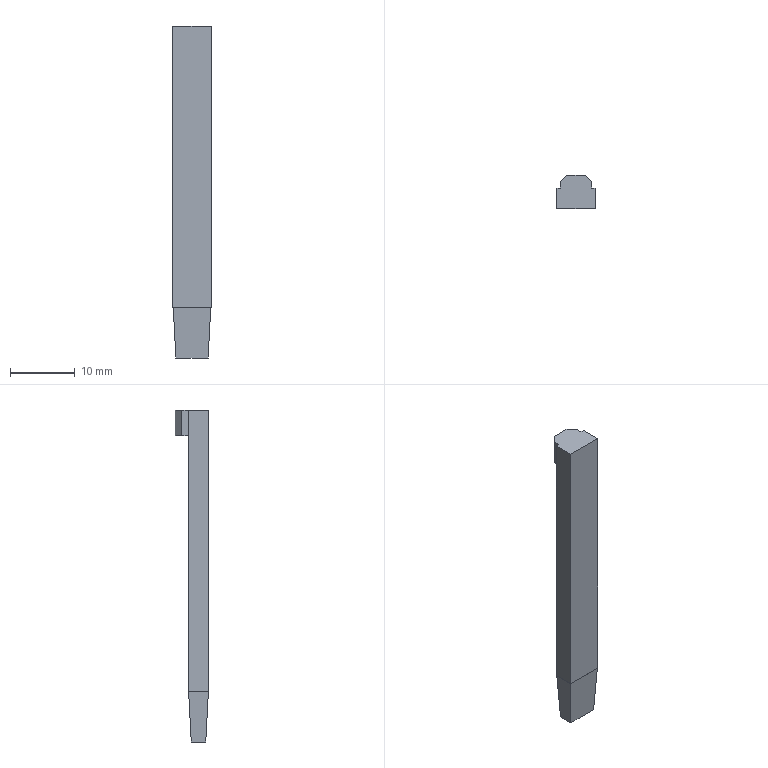Part | Creo | 1 solid | 21 faces | box 5.891 x 5.155 x 51.155 mm | volume 951.101 mm3 | plane 21
STEP:
#1=CARTESIAN_POINT('',(0.,0.,0.));
#2=DIRECTION('',(0.,0.,1.));
#3=DIRECTION('',(1.,0.,0.));
#4=AXIS2_PLACEMENT_3D('',#1,#2,#3);
#5=CARTESIAN_POINT('',(-32.42,12.973,85.91));
#6=VERTEX_POINT('',#5);
#7=CARTESIAN_POINT('',(-32.42,12.973,42.593));
#8=VERTEX_POINT('',#7);
#9=CARTESIAN_POINT('',(-32.42,12.973,85.91));
#10=DIRECTION('',(0.,0.,-1.));
#11=VECTOR('',#10,43.316);
#12=LINE('',#9,#11);
#13=EDGE_CURVE('',#6,#8,#12,.T.);
#14=ORIENTED_EDGE('',*,*,#13,.F.);
#15=CARTESIAN_POINT('',(-26.529,12.973,85.91));
#16=VERTEX_POINT('',#15);
#17=CARTESIAN_POINT('',(-32.42,12.973,85.91));
#18=DIRECTION('',(1.,0.,0.));
#19=VECTOR('',#18,5.891);
#20=LINE('',#17,#19);
#21=EDGE_CURVE('',#6,#16,#20,.T.);
#22=ORIENTED_EDGE('',*,*,#21,.T.);
#23=CARTESIAN_POINT('',(-26.529,12.973,42.593));
#24=VERTEX_POINT('',#23);
#25=CARTESIAN_POINT('',(-26.529,12.973,85.91));
#26=DIRECTION('',(0.,0.,-1.));
#27=VECTOR('',#26,43.316);
#28=LINE('',#25,#27);
#29=EDGE_CURVE('',#16,#24,#28,.T.);
#30=ORIENTED_EDGE('',*,*,#29,.T.);
#31=CARTESIAN_POINT('',(-26.529,12.973,42.593));
#32=DIRECTION('',(-1.,0.,0.));
#33=VECTOR('',#32,5.891);
#34=LINE('',#31,#33);
#35=EDGE_CURVE('',#24,#8,#34,.T.);
#36=ORIENTED_EDGE('',*,*,#35,.T.);
#37=EDGE_LOOP('',(#14,#22,#30,#36));
#38=FACE_OUTER_BOUND('',#37,.F.);
#39=CARTESIAN_POINT('',(-29.474,12.973,14.755));
#40=DIRECTION('',(0.,-1.,0.));
#41=DIRECTION('',(0.,0.,-1.));
#42=AXIS2_PLACEMENT_3D('',#39,#40,#41);
#43=PLANE('',#42);
#44=ADVANCED_FACE('',(#38),#43,.T.);
#45=CARTESIAN_POINT('',(-32.42,16.128,85.91));
#46=VERTEX_POINT('',#45);
#47=CARTESIAN_POINT('',(-32.42,16.128,42.593));
#48=VERTEX_POINT('',#47);
#49=CARTESIAN_POINT('',(-32.42,16.128,85.91));
#50=DIRECTION('',(0.,0.,-1.));
#51=VECTOR('',#50,43.316);
#52=LINE('',#49,#51);
#53=EDGE_CURVE('',#46,#48,#52,.T.);
#54=ORIENTED_EDGE('',*,*,#53,.F.);
#55=CARTESIAN_POINT('',(-32.42,16.128,85.91));
#56=DIRECTION('',(0.,-1.,0.));
#57=VECTOR('',#56,3.155);
#58=LINE('',#55,#57);
#59=EDGE_CURVE('',#46,#6,#58,.T.);
#60=ORIENTED_EDGE('',*,*,#59,.T.);
#61=ORIENTED_EDGE('',*,*,#13,.T.);
#62=CARTESIAN_POINT('',(-32.42,12.973,42.593));
#63=DIRECTION('',(0.,1.,0.));
#64=VECTOR('',#63,3.155);
#65=LINE('',#62,#64);
#66=EDGE_CURVE('',#8,#48,#65,.T.);
#67=ORIENTED_EDGE('',*,*,#66,.T.);
#68=EDGE_LOOP('',(#54,#60,#61,#67));
#69=FACE_OUTER_BOUND('',#68,.F.);
#70=CARTESIAN_POINT('',(-32.42,14.551,14.755));
#71=DIRECTION('',(-1.,0.,0.));
#72=DIRECTION('',(0.,0.,1.));
#73=AXIS2_PLACEMENT_3D('',#70,#71,#72);
#74=PLANE('',#73);
#75=ADVANCED_FACE('',(#69),#74,.T.);
#76=CARTESIAN_POINT('',(-26.529,16.128,85.91));
#77=VERTEX_POINT('',#76);
#78=CARTESIAN_POINT('',(-26.529,16.128,42.593));
#79=VERTEX_POINT('',#78);
#80=CARTESIAN_POINT('',(-26.529,16.128,85.91));
#81=DIRECTION('',(0.,0.,-1.));
#82=VECTOR('',#81,43.316);
#83=LINE('',#80,#82);
#84=EDGE_CURVE('',#77,#79,#83,.T.);
#85=ORIENTED_EDGE('',*,*,#84,.F.);
#86=CARTESIAN_POINT('',(-27.079,16.128,85.91));
#87=VERTEX_POINT('',#86);
#88=CARTESIAN_POINT('',(-26.529,16.128,85.91));
#89=DIRECTION('',(-1.,0.,0.));
#90=VECTOR('',#89,0.55);
#91=LINE('',#88,#90);
#92=EDGE_CURVE('',#77,#87,#91,.T.);
#93=ORIENTED_EDGE('',*,*,#92,.T.);
#94=CARTESIAN_POINT('',(-27.079,16.128,81.91));
#95=VERTEX_POINT('',#94);
#96=CARTESIAN_POINT('',(-27.079,16.128,81.91));
#97=DIRECTION('',(0.,0.,1.));
#98=VECTOR('',#97,4.);
#99=LINE('',#96,#98);
#100=EDGE_CURVE('',#95,#87,#99,.T.);
#101=ORIENTED_EDGE('',*,*,#100,.F.);
#102=CARTESIAN_POINT('',(-31.87,16.128,81.91));
#103=VERTEX_POINT('',#102);
#104=CARTESIAN_POINT('',(-31.87,16.128,81.91));
#105=DIRECTION('',(1.,0.,0.));
#106=VECTOR('',#105,4.791);
#107=LINE('',#104,#106);
#108=EDGE_CURVE('',#103,#95,#107,.T.);
#109=ORIENTED_EDGE('',*,*,#108,.F.);
#110=CARTESIAN_POINT('',(-31.87,16.128,85.91));
#111=VERTEX_POINT('',#110);
#112=CARTESIAN_POINT('',(-31.87,16.128,85.91));
#113=DIRECTION('',(0.,0.,-1.));
#114=VECTOR('',#113,4.);
#115=LINE('',#112,#114);
#116=EDGE_CURVE('',#111,#103,#115,.T.);
#117=ORIENTED_EDGE('',*,*,#116,.F.);
#118=CARTESIAN_POINT('',(-31.87,16.128,85.91));
#119=DIRECTION('',(-1.,0.,0.));
#120=VECTOR('',#119,0.55);
#121=LINE('',#118,#120);
#122=EDGE_CURVE('',#111,#46,#121,.T.);
#123=ORIENTED_EDGE('',*,*,#122,.T.);
#124=ORIENTED_EDGE('',*,*,#53,.T.);
#125=CARTESIAN_POINT('',(-32.42,16.128,42.593));
#126=DIRECTION('',(1.,0.,0.));
#127=VECTOR('',#126,5.891);
#128=LINE('',#125,#127);
#129=EDGE_CURVE('',#48,#79,#128,.T.);
#130=ORIENTED_EDGE('',*,*,#129,.T.);
#131=EDGE_LOOP('',(#85,#93,#101,#109,#117,#123,#124,#130));
#132=FACE_OUTER_BOUND('',#131,.F.);
#133=CARTESIAN_POINT('',(-29.474,16.128,14.755));
#134=DIRECTION('',(0.,1.,0.));
#135=DIRECTION('',(0.,0.,1.));
#136=AXIS2_PLACEMENT_3D('',#133,#134,#135);
#137=PLANE('',#136);
#138=ADVANCED_FACE('',(#132),#137,.T.);
#139=ORIENTED_EDGE('',*,*,#29,.F.);
#140=CARTESIAN_POINT('',(-26.529,12.973,85.91));
#141=DIRECTION('',(0.,1.,0.));
#142=VECTOR('',#141,3.155);
#143=LINE('',#140,#142);
#144=EDGE_CURVE('',#16,#77,#143,.T.);
#145=ORIENTED_EDGE('',*,*,#144,.T.);
#146=ORIENTED_EDGE('',*,*,#84,.T.);
#147=CARTESIAN_POINT('',(-26.529,16.128,42.593));
#148=DIRECTION('',(0.,-1.,0.));
#149=VECTOR('',#148,3.155);
#150=LINE('',#147,#149);
#151=EDGE_CURVE('',#79,#24,#150,.T.);
#152=ORIENTED_EDGE('',*,*,#151,.T.);
#153=EDGE_LOOP('',(#139,#145,#146,#152));
#154=FACE_OUTER_BOUND('',#153,.F.);
#155=CARTESIAN_POINT('',(-26.529,14.551,14.755));
#156=DIRECTION('',(1.,0.,0.));
#157=DIRECTION('',(0.,0.,-1.));
#158=AXIS2_PLACEMENT_3D('',#155,#156,#157);
#159=PLANE('',#158);
#160=ADVANCED_FACE('',(#154),#159,.T.);
#161=CARTESIAN_POINT('',(-27.079,17.128,85.91));
#162=VERTEX_POINT('',#161);
#163=CARTESIAN_POINT('',(-27.079,16.128,85.91));
#164=DIRECTION('',(0.,1.,0.));
#165=VECTOR('',#164,1.);
#166=LINE('',#163,#165);
#167=EDGE_CURVE('',#87,#162,#166,.T.);
#168=ORIENTED_EDGE('',*,*,#167,.F.);
#169=ORIENTED_EDGE('',*,*,#92,.F.);
#170=ORIENTED_EDGE('',*,*,#144,.F.);
#171=ORIENTED_EDGE('',*,*,#21,.F.);
#172=ORIENTED_EDGE('',*,*,#59,.F.);
#173=ORIENTED_EDGE('',*,*,#122,.F.);
#174=CARTESIAN_POINT('',(-31.87,17.128,85.91));
#175=VERTEX_POINT('',#174);
#176=CARTESIAN_POINT('',(-31.87,17.128,85.91));
#177=DIRECTION('',(0.,-1.,0.));
#178=VECTOR('',#177,1.);
#179=LINE('',#176,#178);
#180=EDGE_CURVE('',#175,#111,#179,.T.);
#181=ORIENTED_EDGE('',*,*,#180,.F.);
#182=CARTESIAN_POINT('',(-30.87,18.128,85.91));
#183=VERTEX_POINT('',#182);
#184=CARTESIAN_POINT('',(-30.87,18.128,85.91));
#185=DIRECTION('',(-0.7071,-0.7071,0.));
#186=VECTOR('',#185,1.414);
#187=LINE('',#184,#186);
#188=EDGE_CURVE('',#183,#175,#187,.T.);
#189=ORIENTED_EDGE('',*,*,#188,.F.);
#190=CARTESIAN_POINT('',(-28.079,18.128,85.91));
#191=VERTEX_POINT('',#190);
#192=CARTESIAN_POINT('',(-28.079,18.128,85.91));
#193=DIRECTION('',(-1.,0.,0.));
#194=VECTOR('',#193,2.791);
#195=LINE('',#192,#194);
#196=EDGE_CURVE('',#191,#183,#195,.T.);
#197=ORIENTED_EDGE('',*,*,#196,.F.);
#198=CARTESIAN_POINT('',(-27.079,17.128,85.91));
#199=DIRECTION('',(-0.7071,0.7071,0.));
#200=VECTOR('',#199,1.414);
#201=LINE('',#198,#200);
#202=EDGE_CURVE('',#162,#191,#201,.T.);
#203=ORIENTED_EDGE('',*,*,#202,.F.);
#204=EDGE_LOOP('',(#168,#169,#170,#171,#172,#173,#181,#189,#197,#203));
#205=FACE_OUTER_BOUND('',#204,.F.);
#206=CARTESIAN_POINT('',(62.144,-0.4125,85.91));
#207=DIRECTION('',(0.,0.,1.));
#208=DIRECTION('',(0.,1.,0.));
#209=AXIS2_PLACEMENT_3D('',#206,#207,#208);
#210=PLANE('',#209);
#211=ADVANCED_FACE('',(#205),#210,.T.);
#212=CARTESIAN_POINT('',(-27.079,17.128,81.91));
#213=VERTEX_POINT('',#212);
#214=CARTESIAN_POINT('',(-27.079,17.128,81.91));
#215=DIRECTION('',(0.,-1.,0.));
#216=VECTOR('',#215,1.);
#217=LINE('',#214,#216);
#218=EDGE_CURVE('',#213,#95,#217,.T.);
#219=ORIENTED_EDGE('',*,*,#218,.T.);
#220=ORIENTED_EDGE('',*,*,#100,.T.);
#221=ORIENTED_EDGE('',*,*,#167,.T.);
#222=CARTESIAN_POINT('',(-27.079,17.128,85.91));
#223=DIRECTION('',(0.,0.,-1.));
#224=VECTOR('',#223,4.);
#225=LINE('',#222,#224);
#226=EDGE_CURVE('',#162,#213,#225,.T.);
#227=ORIENTED_EDGE('',*,*,#226,.T.);
#228=EDGE_LOOP('',(#219,#220,#221,#227));
#229=FACE_OUTER_BOUND('',#228,.F.);
#230=CARTESIAN_POINT('',(-27.079,16.578,81.91));
#231=DIRECTION('',(1.,0.,0.));
#232=DIRECTION('',(0.,0.,-1.));
#233=AXIS2_PLACEMENT_3D('',#230,#231,#232);
#234=PLANE('',#233);
#235=ADVANCED_FACE('',(#229),#234,.T.);
#236=CARTESIAN_POINT('',(-30.87,18.128,81.91));
#237=VERTEX_POINT('',#236);
#238=CARTESIAN_POINT('',(-28.079,18.128,81.91));
#239=VERTEX_POINT('',#238);
#240=CARTESIAN_POINT('',(-30.87,18.128,81.91));
#241=DIRECTION('',(1.,0.,0.));
#242=VECTOR('',#241,2.791);
#243=LINE('',#240,#242);
#244=EDGE_CURVE('',#237,#239,#243,.T.);
#245=ORIENTED_EDGE('',*,*,#244,.F.);
#246=CARTESIAN_POINT('',(-31.87,17.128,81.91));
#247=VERTEX_POINT('',#246);
#248=CARTESIAN_POINT('',(-31.87,17.128,81.91));
#249=DIRECTION('',(0.7071,0.7071,0.));
#250=VECTOR('',#249,1.414);
#251=LINE('',#248,#250);
#252=EDGE_CURVE('',#247,#237,#251,.T.);
#253=ORIENTED_EDGE('',*,*,#252,.F.);
#254=CARTESIAN_POINT('',(-31.87,16.128,81.91));
#255=DIRECTION('',(0.,1.,0.));
#256=VECTOR('',#255,1.);
#257=LINE('',#254,#256);
#258=EDGE_CURVE('',#103,#247,#257,.T.);
#259=ORIENTED_EDGE('',*,*,#258,.F.);
#260=ORIENTED_EDGE('',*,*,#108,.T.);
#261=ORIENTED_EDGE('',*,*,#218,.F.);
#262=CARTESIAN_POINT('',(-28.079,18.128,81.91));
#263=DIRECTION('',(0.7071,-0.7071,0.));
#264=VECTOR('',#263,1.414);
#265=LINE('',#262,#264);
#266=EDGE_CURVE('',#239,#213,#265,.T.);
#267=ORIENTED_EDGE('',*,*,#266,.F.);
#268=EDGE_LOOP('',(#245,#253,#259,#260,#261,#267));
#269=FACE_OUTER_BOUND('',#268,.F.);
#270=CARTESIAN_POINT('',(-29.474,16.578,81.91));
#271=DIRECTION('',(0.,0.,-1.));
#272=DIRECTION('',(-1.,0.,0.));
#273=AXIS2_PLACEMENT_3D('',#270,#271,#272);
#274=PLANE('',#273);
#275=ADVANCED_FACE('',(#269),#274,.T.);
#276=ORIENTED_EDGE('',*,*,#196,.T.);
#277=CARTESIAN_POINT('',(-30.87,18.128,85.91));
#278=DIRECTION('',(0.,0.,-1.));
#279=VECTOR('',#278,4.);
#280=LINE('',#277,#279);
#281=EDGE_CURVE('',#183,#237,#280,.T.);
#282=ORIENTED_EDGE('',*,*,#281,.T.);
#283=ORIENTED_EDGE('',*,*,#244,.T.);
#284=CARTESIAN_POINT('',(-28.079,18.128,81.91));
#285=DIRECTION('',(0.,0.,1.));
#286=VECTOR('',#285,4.);
#287=LINE('',#284,#286);
#288=EDGE_CURVE('',#239,#191,#287,.T.);
#289=ORIENTED_EDGE('',*,*,#288,.T.);
#290=EDGE_LOOP('',(#276,#282,#283,#289));
#291=FACE_OUTER_BOUND('',#290,.F.);
#292=CARTESIAN_POINT('',(-29.474,18.128,81.91));
#293=DIRECTION('',(0.,1.,0.));
#294=DIRECTION('',(0.,0.,1.));
#295=AXIS2_PLACEMENT_3D('',#292,#293,#294);
#296=PLANE('',#295);
#297=ADVANCED_FACE('',(#291),#296,.T.);
#298=ORIENTED_EDGE('',*,*,#252,.T.);
#299=ORIENTED_EDGE('',*,*,#281,.F.);
#300=ORIENTED_EDGE('',*,*,#188,.T.);
#301=CARTESIAN_POINT('',(-31.87,17.128,81.91));
#302=DIRECTION('',(0.,0.,1.));
#303=VECTOR('',#302,4.);
#304=LINE('',#301,#303);
#305=EDGE_CURVE('',#247,#175,#304,.T.);
#306=ORIENTED_EDGE('',*,*,#305,.F.);
#307=EDGE_LOOP('',(#298,#299,#300,#306));
#308=FACE_OUTER_BOUND('',#307,.F.);
#309=CARTESIAN_POINT('',(-30.87,18.128,81.91));
#310=DIRECTION('',(0.7071,-0.7071,0.));
#311=DIRECTION('',(0.,0.,1.));
#312=AXIS2_PLACEMENT_3D('',#309,#310,#311);
#313=PLANE('',#312);
#314=ADVANCED_FACE('',(#308),#313,.F.);
#315=ORIENTED_EDGE('',*,*,#180,.T.);
#316=ORIENTED_EDGE('',*,*,#116,.T.);
#317=ORIENTED_EDGE('',*,*,#258,.T.);
#318=ORIENTED_EDGE('',*,*,#305,.T.);
#319=EDGE_LOOP('',(#315,#316,#317,#318));
#320=FACE_OUTER_BOUND('',#319,.F.);
#321=CARTESIAN_POINT('',(-31.87,16.578,81.91));
#322=DIRECTION('',(-1.,0.,0.));
#323=DIRECTION('',(0.,0.,1.));
#324=AXIS2_PLACEMENT_3D('',#321,#322,#323);
#325=PLANE('',#324);
#326=ADVANCED_FACE('',(#320),#325,.T.);
#327=ORIENTED_EDGE('',*,*,#266,.T.);
#328=ORIENTED_EDGE('',*,*,#226,.F.);
#329=ORIENTED_EDGE('',*,*,#202,.T.);
#330=ORIENTED_EDGE('',*,*,#288,.F.);
#331=EDGE_LOOP('',(#327,#328,#329,#330));
#332=FACE_OUTER_BOUND('',#331,.F.);
#333=CARTESIAN_POINT('',(-27.079,17.128,81.91));
#334=DIRECTION('',(-0.7071,-0.7071,0.));
#335=DIRECTION('',(0.,0.,1.));
#336=AXIS2_PLACEMENT_3D('',#333,#334,#335);
#337=PLANE('',#336);
#338=ADVANCED_FACE('',(#332),#337,.F.);
#339=ORIENTED_EDGE('',*,*,#151,.F.);
#340=ORIENTED_EDGE('',*,*,#129,.F.);
#341=ORIENTED_EDGE('',*,*,#66,.F.);
#342=ORIENTED_EDGE('',*,*,#35,.F.);
#343=EDGE_LOOP('',(#339,#340,#341,#342));
#344=FACE_OUTER_BOUND('',#343,.F.);
#345=CARTESIAN_POINT('',(-32.37,13.023,42.593));
#346=VERTEX_POINT('',#345);
#347=CARTESIAN_POINT('',(-26.579,13.023,42.593));
#348=VERTEX_POINT('',#347);
#349=CARTESIAN_POINT('',(-32.37,13.023,42.593));
#350=DIRECTION('',(1.,0.,0.));
#351=VECTOR('',#350,5.791);
#352=LINE('',#349,#351);
#353=EDGE_CURVE('',#346,#348,#352,.T.);
#354=ORIENTED_EDGE('',*,*,#353,.F.);
#355=CARTESIAN_POINT('',(-32.37,16.078,42.593));
#356=VERTEX_POINT('',#355);
#357=CARTESIAN_POINT('',(-32.37,13.023,42.593));
#358=DIRECTION('',(0.,1.,0.));
#359=VECTOR('',#358,3.055);
#360=LINE('',#357,#359);
#361=EDGE_CURVE('',#346,#356,#360,.T.);
#362=ORIENTED_EDGE('',*,*,#361,.T.);
#363=CARTESIAN_POINT('',(-26.579,16.078,42.593));
#364=VERTEX_POINT('',#363);
#365=CARTESIAN_POINT('',(-32.37,16.078,42.593));
#366=DIRECTION('',(1.,0.,0.));
#367=VECTOR('',#366,5.791);
#368=LINE('',#365,#367);
#369=EDGE_CURVE('',#356,#364,#368,.T.);
#370=ORIENTED_EDGE('',*,*,#369,.T.);
#371=CARTESIAN_POINT('',(-26.579,16.078,42.593));
#372=DIRECTION('',(0.,-1.,0.));
#373=VECTOR('',#372,3.055);
#374=LINE('',#371,#373);
#375=EDGE_CURVE('',#364,#348,#374,.T.);
#376=ORIENTED_EDGE('',*,*,#375,.T.);
#377=EDGE_LOOP('',(#354,#362,#370,#376));
#378=FACE_BOUND('',#377,.F.);
#379=CARTESIAN_POINT('',(-26.579,16.078,42.593));
#380=DIRECTION('',(0.,0.,1.));
#381=DIRECTION('',(1.,0.,0.));
#382=AXIS2_PLACEMENT_3D('',#379,#380,#381);
#383=PLANE('',#382);
#384=ADVANCED_FACE('',(#344,#378),#383,.F.);
#385=CARTESIAN_POINT('',(-31.959,13.434,34.755));
#386=VERTEX_POINT('',#385);
#387=CARTESIAN_POINT('',(-32.37,13.023,42.593));
#388=DIRECTION('',(0.05226,0.05226,-0.9973));
#389=VECTOR('',#388,7.861);
#390=LINE('',#387,#389);
#391=EDGE_CURVE('',#346,#386,#390,.T.);
#392=ORIENTED_EDGE('',*,*,#391,.F.);
#393=ORIENTED_EDGE('',*,*,#353,.T.);
#394=CARTESIAN_POINT('',(-26.99,13.434,34.755));
#395=VERTEX_POINT('',#394);
#396=CARTESIAN_POINT('',(-26.579,13.023,42.593));
#397=DIRECTION('',(-0.05226,0.05226,-0.9973));
#398=VECTOR('',#397,7.861);
#399=LINE('',#396,#398);
#400=EDGE_CURVE('',#348,#395,#399,.T.);
#401=ORIENTED_EDGE('',*,*,#400,.T.);
#402=CARTESIAN_POINT('',(-26.99,13.434,34.755));
#403=DIRECTION('',(-1.,0.,0.));
#404=VECTOR('',#403,4.969);
#405=LINE('',#402,#404);
#406=EDGE_CURVE('',#395,#386,#405,.T.);
#407=ORIENTED_EDGE('',*,*,#406,.T.);
#408=EDGE_LOOP('',(#392,#393,#401,#407));
#409=FACE_OUTER_BOUND('',#408,.F.);
#410=CARTESIAN_POINT('',(-24.101,13.155,40.081));
#411=DIRECTION('',(0.,-0.9986,-0.05234));
#412=DIRECTION('',(1.,0.,0.));
#413=AXIS2_PLACEMENT_3D('',#410,#411,#412);
#414=PLANE('',#413);
#415=ADVANCED_FACE('',(#409),#414,.T.);
#416=CARTESIAN_POINT('',(-31.959,15.668,34.755));
#417=VERTEX_POINT('',#416);
#418=CARTESIAN_POINT('',(-32.37,16.078,42.593));
#419=DIRECTION('',(0.05226,-0.05226,-0.9973));
#420=VECTOR('',#419,7.861);
#421=LINE('',#418,#420);
#422=EDGE_CURVE('',#356,#417,#421,.T.);
#423=ORIENTED_EDGE('',*,*,#422,.F.);
#424=ORIENTED_EDGE('',*,*,#361,.F.);
#425=ORIENTED_EDGE('',*,*,#391,.T.);
#426=CARTESIAN_POINT('',(-31.959,13.434,34.755));
#427=DIRECTION('',(0.,1.,0.));
#428=VECTOR('',#427,2.233);
#429=LINE('',#426,#428);
#430=EDGE_CURVE('',#386,#417,#429,.T.);
#431=ORIENTED_EDGE('',*,*,#430,.T.);
#432=EDGE_LOOP('',(#423,#424,#425,#431));
#433=FACE_OUTER_BOUND('',#432,.F.);
#434=CARTESIAN_POINT('',(-32.238,10.545,40.081));
#435=DIRECTION('',(-0.9986,0.,-0.05234));
#436=DIRECTION('',(0.,-1.,0.));
#437=AXIS2_PLACEMENT_3D('',#434,#435,#436);
#438=PLANE('',#437);
#439=ADVANCED_FACE('',(#433),#438,.T.);
#440=CARTESIAN_POINT('',(-31.233,15.67,34.804));
#441=VERTEX_POINT('',#440);
#442=CARTESIAN_POINT('',(-27.716,15.67,34.804));
#443=VERTEX_POINT('',#442);
#444=CARTESIAN_POINT('',(-31.233,15.67,34.804));
#445=DIRECTION('',(1.,0.,0.));
#446=VECTOR('',#445,3.517);
#447=LINE('',#444,#446);
#448=EDGE_CURVE('',#441,#443,#447,.T.);
#449=ORIENTED_EDGE('',*,*,#448,.T.);
#450=CARTESIAN_POINT('',(-27.716,15.668,34.755));
#451=VERTEX_POINT('',#450);
#452=CARTESIAN_POINT('',(-27.716,15.67,34.804));
#453=DIRECTION('',(0.,-0.05234,-0.9986));
#454=VECTOR('',#453,0.05007);
#455=LINE('',#452,#454);
#456=EDGE_CURVE('',#443,#451,#455,.T.);
#457=ORIENTED_EDGE('',*,*,#456,.T.);
#458=CARTESIAN_POINT('',(-26.99,15.668,34.755));
#459=VERTEX_POINT('',#458);
#460=CARTESIAN_POINT('',(-27.716,15.668,34.755));
#461=DIRECTION('',(1.,0.,0.));
#462=VECTOR('',#461,0.7259);
#463=LINE('',#460,#462);
#464=EDGE_CURVE('',#451,#459,#463,.T.);
#465=ORIENTED_EDGE('',*,*,#464,.T.);
#466=CARTESIAN_POINT('',(-26.579,16.078,42.593));
#467=DIRECTION('',(-0.05226,-0.05226,-0.9973));
#468=VECTOR('',#467,7.861);
#469=LINE('',#466,#468);
#470=EDGE_CURVE('',#364,#459,#469,.T.);
#471=ORIENTED_EDGE('',*,*,#470,.F.);
#472=ORIENTED_EDGE('',*,*,#369,.F.);
#473=ORIENTED_EDGE('',*,*,#422,.T.);
#474=CARTESIAN_POINT('',(-31.233,15.668,34.755));
#475=VERTEX_POINT('',#474);
#476=CARTESIAN_POINT('',(-31.959,15.668,34.755));
#477=DIRECTION('',(1.,0.,0.));
#478=VECTOR('',#477,0.7259);
#479=LINE('',#476,#478);
#480=EDGE_CURVE('',#417,#475,#479,.T.);
#481=ORIENTED_EDGE('',*,*,#480,.T.);
#482=CARTESIAN_POINT('',(-31.233,15.668,34.755));
#483=DIRECTION('',(0.,0.05234,0.9986));
#484=VECTOR('',#483,0.05007);
#485=LINE('',#482,#484);
#486=EDGE_CURVE('',#475,#441,#485,.T.);
#487=ORIENTED_EDGE('',*,*,#486,.T.);
#488=EDGE_LOOP('',(#449,#457,#465,#471,#472,#473,#481,#487));
#489=FACE_OUTER_BOUND('',#488,.F.);
#490=CARTESIAN_POINT('',(-24.101,15.668,34.755));
#491=DIRECTION('',(0.,-0.9986,0.05234));
#492=DIRECTION('',(-1.,0.,0.));
#493=AXIS2_PLACEMENT_3D('',#490,#491,#492);
#494=PLANE('',#493);
#495=ADVANCED_FACE('',(#489),#494,.F.);
#496=CARTESIAN_POINT('',(-27.716,14.27,34.804));
#497=VERTEX_POINT('',#496);
#498=CARTESIAN_POINT('',(-27.716,15.67,34.804));
#499=DIRECTION('',(0.,-1.,0.));
#500=VECTOR('',#499,1.4);
#501=LINE('',#498,#500);
#502=EDGE_CURVE('',#443,#497,#501,.T.);
#503=ORIENTED_EDGE('',*,*,#502,.F.);
#504=ORIENTED_EDGE('',*,*,#448,.F.);
#505=CARTESIAN_POINT('',(-31.233,14.27,34.804));
#506=VERTEX_POINT('',#505);
#507=CARTESIAN_POINT('',(-31.233,14.27,34.804));
#508=DIRECTION('',(0.,1.,0.));
#509=VECTOR('',#508,1.4);
#510=LINE('',#507,#509);
#511=EDGE_CURVE('',#506,#441,#510,.T.);
#512=ORIENTED_EDGE('',*,*,#511,.F.);
#513=CARTESIAN_POINT('',(-27.716,14.27,34.804));
#514=DIRECTION('',(-1.,0.,0.));
#515=VECTOR('',#514,3.517);
#516=LINE('',#513,#515);
#517=EDGE_CURVE('',#497,#506,#516,.T.);
#518=ORIENTED_EDGE('',*,*,#517,.F.);
#519=EDGE_LOOP('',(#503,#504,#512,#518));
#520=FACE_OUTER_BOUND('',#519,.F.);
#521=CARTESIAN_POINT('',(-0.07825,-88.35,34.804));
#522=DIRECTION('',(0.,0.,-1.));
#523=DIRECTION('',(0.,-1.,0.));
#524=AXIS2_PLACEMENT_3D('',#521,#522,#523);
#525=PLANE('',#524);
#526=ADVANCED_FACE('',(#520),#525,.T.);
#527=CARTESIAN_POINT('',(-27.716,14.27,34.755));
#528=VERTEX_POINT('',#527);
#529=CARTESIAN_POINT('',(-27.716,14.27,34.755));
#530=DIRECTION('',(0.,1.,0.));
#531=VECTOR('',#530,1.397);
#532=LINE('',#529,#531);
#533=EDGE_CURVE('',#528,#451,#532,.T.);
#534=ORIENTED_EDGE('',*,*,#533,.T.);
#535=ORIENTED_EDGE('',*,*,#456,.F.);
#536=ORIENTED_EDGE('',*,*,#502,.T.);
#537=CARTESIAN_POINT('',(-27.716,14.27,34.755));
#538=DIRECTION('',(0.,0.,1.));
#539=VECTOR('',#538,0.05);
#540=LINE('',#537,#539);
#541=EDGE_CURVE('',#528,#497,#540,.T.);
#542=ORIENTED_EDGE('',*,*,#541,.F.);
#543=EDGE_LOOP('',(#534,#535,#536,#542));
#544=FACE_OUTER_BOUND('',#543,.F.);
#545=CARTESIAN_POINT('',(-27.716,15.668,34.255));
#546=DIRECTION('',(-1.,0.,0.));
#547=DIRECTION('',(0.,0.,1.));
#548=AXIS2_PLACEMENT_3D('',#545,#546,#547);
#549=PLANE('',#548);
#550=ADVANCED_FACE('',(#544),#549,.T.);
#551=CARTESIAN_POINT('',(-31.233,14.27,34.755));
#552=VERTEX_POINT('',#551);
#553=CARTESIAN_POINT('',(-31.233,15.668,34.755));
#554=DIRECTION('',(0.,-1.,0.));
#555=VECTOR('',#554,1.397);
#556=LINE('',#553,#555);
#557=EDGE_CURVE('',#475,#552,#556,.T.);
#558=ORIENTED_EDGE('',*,*,#557,.F.);
#559=ORIENTED_EDGE('',*,*,#480,.F.);
#560=ORIENTED_EDGE('',*,*,#430,.F.);
#561=ORIENTED_EDGE('',*,*,#406,.F.);
#562=CARTESIAN_POINT('',(-26.99,15.668,34.755));
#563=DIRECTION('',(0.,-1.,0.));
#564=VECTOR('',#563,2.233);
#565=LINE('',#562,#564);
#566=EDGE_CURVE('',#459,#395,#565,.T.);
#567=ORIENTED_EDGE('',*,*,#566,.F.);
#568=ORIENTED_EDGE('',*,*,#464,.F.);
#569=ORIENTED_EDGE('',*,*,#533,.F.);
#570=CARTESIAN_POINT('',(-31.233,14.27,34.755));
#571=DIRECTION('',(1.,0.,0.));
#572=VECTOR('',#571,3.517);
#573=LINE('',#570,#572);
#574=EDGE_CURVE('',#552,#528,#573,.T.);
#575=ORIENTED_EDGE('',*,*,#574,.F.);
#576=EDGE_LOOP('',(#558,#559,#560,#561,#567,#568,#569,#575));
#577=FACE_OUTER_BOUND('',#576,.F.);
#578=CARTESIAN_POINT('',(-0.07825,-88.35,34.755));
#579=DIRECTION('',(0.,0.,-1.));
#580=DIRECTION('',(0.,-1.,0.));
#581=AXIS2_PLACEMENT_3D('',#578,#579,#580);
#582=PLANE('',#581);
#583=ADVANCED_FACE('',(#577),#582,.T.);
#584=ORIENTED_EDGE('',*,*,#557,.T.);
#585=CARTESIAN_POINT('',(-31.233,14.27,34.755));
#586=DIRECTION('',(0.,0.,1.));
#587=VECTOR('',#586,0.05);
#588=LINE('',#585,#587);
#589=EDGE_CURVE('',#552,#506,#588,.T.);
#590=ORIENTED_EDGE('',*,*,#589,.T.);
#591=ORIENTED_EDGE('',*,*,#511,.T.);
#592=ORIENTED_EDGE('',*,*,#486,.F.);
#593=EDGE_LOOP('',(#584,#590,#591,#592));
#594=FACE_OUTER_BOUND('',#593,.F.);
#595=CARTESIAN_POINT('',(-31.233,14.16,34.255));
#596=DIRECTION('',(1.,0.,0.));
#597=DIRECTION('',(0.,0.,-1.));
#598=AXIS2_PLACEMENT_3D('',#595,#596,#597);
#599=PLANE('',#598);
#600=ADVANCED_FACE('',(#594),#599,.T.);
#601=ORIENTED_EDGE('',*,*,#574,.T.);
#602=ORIENTED_EDGE('',*,*,#541,.T.);
#603=ORIENTED_EDGE('',*,*,#517,.T.);
#604=ORIENTED_EDGE('',*,*,#589,.F.);
#605=EDGE_LOOP('',(#601,#602,#603,#604));
#606=FACE_OUTER_BOUND('',#605,.F.);
#607=CARTESIAN_POINT('',(-0.07825,14.27,34.255));
#608=DIRECTION('',(0.,1.,0.));
#609=DIRECTION('',(0.,0.,1.));
#610=AXIS2_PLACEMENT_3D('',#607,#608,#609);
#611=PLANE('',#610);
#612=ADVANCED_FACE('',(#606),#611,.T.);
#613=ORIENTED_EDGE('',*,*,#400,.F.);
#614=ORIENTED_EDGE('',*,*,#375,.F.);
#615=ORIENTED_EDGE('',*,*,#470,.T.);
#616=ORIENTED_EDGE('',*,*,#566,.T.);
#617=EDGE_LOOP('',(#613,#614,#615,#616));
#618=FACE_OUTER_BOUND('',#617,.F.);
#619=CARTESIAN_POINT('',(-26.711,18.688,40.081));
#620=DIRECTION('',(0.9986,0.,-0.05234));
#621=DIRECTION('',(0.,1.,0.));
#622=AXIS2_PLACEMENT_3D('',#619,#620,#621);
#623=PLANE('',#622);
#624=ADVANCED_FACE('',(#618),#623,.T.);
#625=CLOSED_SHELL('',(#44,#75,#138,#160,#211,#235,#275,#297,#314,#326,#338,#384,#415,#439,#495,#526,#550,#583,#600,#612,#624));
#626=MANIFOLD_SOLID_BREP('',#625);
#627=(LENGTH_UNIT()NAMED_UNIT(*)SI_UNIT(.MILLI.,.METRE.));
#628=UNCERTAINTY_MEASURE_WITH_UNIT(LENGTH_MEASURE(0.005175),#627,'','');
#629=(NAMED_UNIT(*)PLANE_ANGLE_UNIT()SI_UNIT($,.RADIAN.));
#630=PLANE_ANGLE_MEASURE_WITH_UNIT(PLANE_ANGLE_MEASURE(0.01745),#629);
#631=(CONVERSION_BASED_UNIT('DEGREE',#630)NAMED_UNIT(*)PLANE_ANGLE_UNIT());
#632=(NAMED_UNIT(*)SI_UNIT($,.STERADIAN.)SOLID_ANGLE_UNIT());
#633=(GEOMETRIC_REPRESENTATION_CONTEXT(3)GLOBAL_UNCERTAINTY_ASSIGNED_CONTEXT((#628))GLOBAL_UNIT_ASSIGNED_CONTEXT((#627,#631,#632))REPRESENTATION_CONTEXT('',''));
#634=ADVANCED_BREP_SHAPE_REPRESENTATION('',(#4,#626),#633);